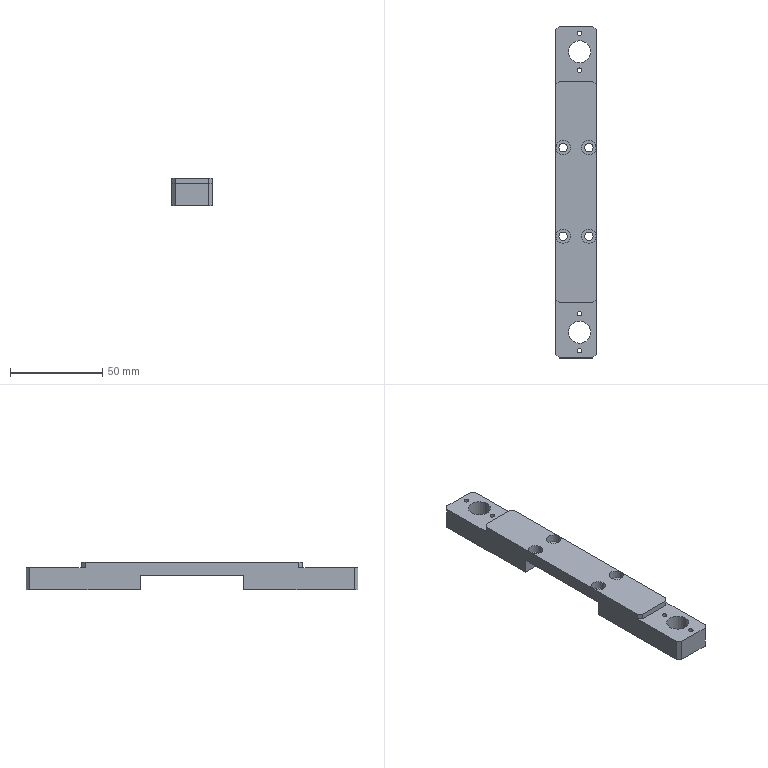CAM job | NX | 3-axis milling, drilling | part box 22 x 180 x 15 mm | stock box 27 x 185 x 20 mm
Tools:
number,name,description,diameter,corner_radius,flute_length,length,flutes
4,D4,平底铣刀-粗,4.0,0.0,25.0,75.0,2
8,D8,平底铣刀-粗,8.0,0.0,30.0,75.0,2
9,D10,平底铣刀-粗,10.0,0.0,35.0,75.0,2
18,D4-J,平底铣刀-精,4.0,0.0,50.0,75.0,2
7,D6-J,平底铣刀-精,6.0,0.0,25.0,75.0,2
10,D10-J,平底铣刀-精,10.0,0.0,35.0,75.0,2
1,D80R0.8飞刀,圆鼻刀-粗,80.0,0.8,50.0,75.0,2
1,D80R0.8飞刀-J,圆鼻刀-精,80.0,0.8,50.0,75.0,2
2,D6倒角刀,倒角刀,6.0,0.0,3.0,25.0,2
20,M3X0.5,丝锥,2.5,0.0,35.0,50.0,2
12,ZT2.5,钻头,2.5,0.0,35.0,50.0,2
11,ZT4.5,钻头,4.5,0.0,35.0,50.0,2
17,ZT10,钻头,10.0,0.0,35.0,50.0,2
Operations:
program,operation,operation_type,tool,method,geometry_group,spindle_rpm,surface_speed,feed_per_tooth,feed_cut,feed_plunge,cut_length_mm,path_length_mm,cut_time_min,machine_time_min
B,底壁铣飞面一刀开粗_COPY,VolumeBased25DMillingOperation,D80R0.8飞刀,分层开粗-切深K-步距G,W-B,2800.0,703.696,0.5357,3000.0,100.0,2593.746,5065.966,0.8646,1.112
B,底壁铣飞面一刀精光_COPY,VolumeBased25DMillingOperation,D80R0.8飞刀-J,侧刃精光-切深K-步距G,W-B,4000.0,1005.28,0.125,1000.0,100.0,287.998,323.998,0.288,0.2916
B,底壁铣分层开粗-中_COPY,VolumeBased25DMillingOperation,D10,分层开粗-切深K-步距G,W-B,8000.0,251.32,0.25,4000.0,100.0,2038.588,2868.773,0.5096,0.5927
B,铣沉头_1,CylinderMilling,D4,METHOD,W-B,8000.0,100.531,0.1125,1800.0,100.0,686.895,939.295,0.3816,0.4068
B,铣孔_1,CylinderMilling,D4-J,METHOD,W-B,8000.0,100.531,0.0375,600.0,100.0,66.763,337.963,0.1113,0.1384
B,钻倒角_2,Operation,D6倒角刀,METHOD,W-B,8000.0,150.796,0.0625,1000.0,0.0,19.0,265.482,0.019,0.0436
B,C0.3平面去毛刺6X45L__COPY_1,SurfaceContour,D6倒角刀,爬面_倒角-切深0-步距G,W-B,8000.0,150.796,0.0938,1500.0,90.0,621.076,1154.276,0.4155,0.4688
B,底壁铣精光底面-中_COPY,VolumeBased25DMillingOperation,D10-J,精光步距切深关,W-B,8000.0,251.32,0.0625,1000.0,100.0,367.77,598.706,0.3678,0.3909
B,底壁铣精光侧面-中-选底面_COPY,VolumeBased25DMillingOperation,D10-J,侧刃精光-切深K-步距G,W-B,8000.0,251.32,0.0625,1000.0,100.0,85.628,245.891,0.0856,0.1017
A,顶面,FaceMilling,D80R0.8飞刀,侧刃精光-切深K-步距G,W-A,4000.0,1005.31,0.125,1000.0,100.0,274.0,310.0,0.274,0.2776
A,外形粗_2,VolumeBased25DMillingOperation,D10,METHOD,W-A,8000.0,251.327,0.3125,5000.0,80.0,9060.031,9113.832,1.812,1.817
A,底壁粗_1,VolumeBased25DMillingOperation,D10,METHOD,W-A,6000.0,113.0,0.2083,3500.0,100.0,4662.4,5009.614,1.332,1.367
A,打点-深0.8,Operation,D6倒角刀,NONE,W-A,8000.0,150.796,0.0312,500.0,90.0,18.0,287.397,0.036,0.0629
A,通孔-M3螺纹底孔,Operation,ZT2.5,NONE,W-A,3000.0,23.562,0.05,300.0,90.0,75.004,365.062,0.25,0.279
A,通孔-5-6,Operation,ZT4.5,NONE,W-A,3000.0,42.411,0.025,150.0,90.0,27.808,190.697,0.1854,0.2017
A,通孔-精孔12.0预钻,Operation,ZT10,NONE,W-A,800.0,29.657,0.125,200.0,90.0,35.009,263.021,0.175,0.1978
A,铣孔开粗D8_1,CylinderMilling,D8,NONE,W-A,8000.0,201.062,0.075,1200.0,100.0,565.414,821.414,0.4712,0.4968
A,底精_1,VolumeBased25DMillingOperation,D6-J,METHOD,W-A,6000.0,113.0,0.2083,1200.0,100.0,421.099,476.099,0.3509,0.3564
A,钻倒角_1,Operation,D6倒角刀,METHOD,W-A,8000.0,150.796,0.0312,500.0,0.0,19.0,259.482,0.038,0.062
A,C0.3平面去毛刺6X45L__COPY,SurfaceContour,D6倒角刀,爬面_倒角-切深0-步距G,W-A,8000.0,150.796,0.0938,1500.0,90.0,635.72,1183.616,0.4277,0.4825
A,通孔-攻牙M3,Operation,M3X0.5,METHOD,W-A,800.0,6.283,0.0003,0.5,90.0,64.0,343.054,128.0,128.028
A,底壁铣精光侧面-中_COPY,VolumeBased25DMillingOperation,D6-J,侧刃精光-切深K-步距G,W-A,6000.0,113.097,0.05,600.0,100.0,104.015,339.449,0.1734,0.1969
A,底侧精_3,VolumeBased25DMillingOperation,D6-J,METHOD,W-A,6000.0,113.0,0.1,1200.0,100.0,63.483,221.403,0.0529,0.0687
A,外形半精_2,VolumeBased25DMillingOperation,D10-J,METHOD,W-A,8000.0,251.327,0.0625,1000.0,100.0,435.688,505.288,0.4357,0.4426